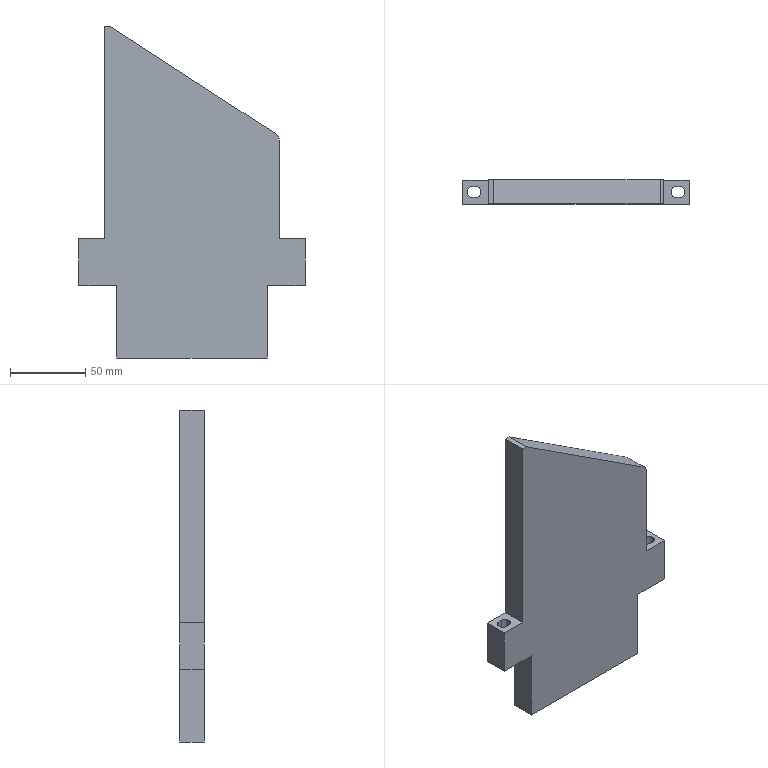Part | STEP file | 1 solid | 32 faces | box 150 x 16 x 219.952 mm | volume 343529 mm3 | plane 23 | cylinder 9 | commonest cylinder face diameters 6 x8 10 x1